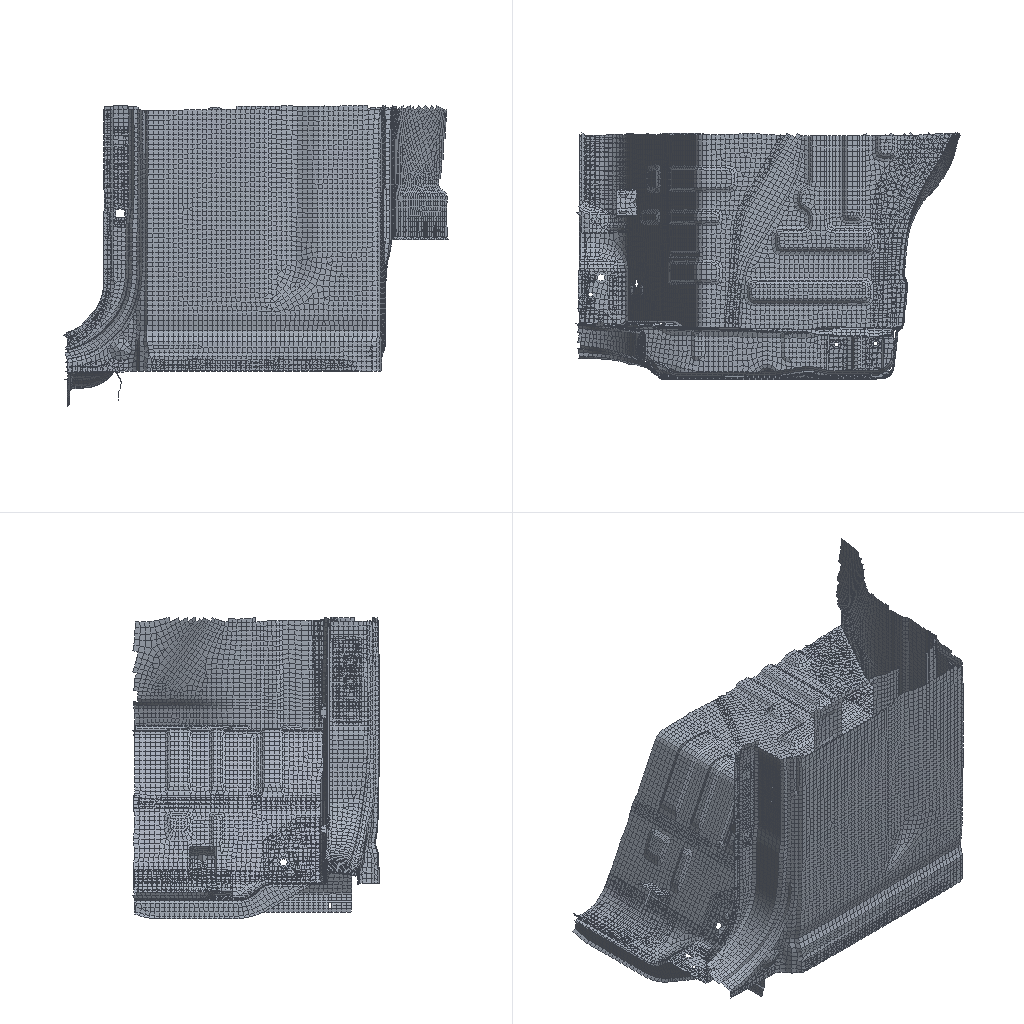Simulation study | nastran
Set-up summary:
category,name,step,type,value,unit,region
solver,nx_nastran
units,not stated in the deck,,not stated
analysis,deck,,static,static
analysis,solution,,SOL,101
load_step,SUBCASE 2,2,SUBCASE,SPC=2 LOAD=5
load_step,SUBCASE 3,3,SUBCASE,SPC=2 LOAD=4
load_step,SUBCASE 4,4,SUBCASE,SPC=2 LOAD=3
load_step,requested,,,3
mesh,nodes,,,25501
mesh,elements,,,22783
element_type,CHEXA,,unverified,187
element_type,CQUAD4,,shell,22113
element_type,CTRIA3,,shell,670
load,load commands in deck,,count,3
bc,support commands in deck,,count,620
check,setup vs results,,match,"every grid point's frame and coordinates and every element id; grid points of CHEXA, CQUAD4, CTRIA3 elements"
Nastran input file, long lists of numbers shortened:
$$------------------------------------------------------------------------------$
$$                                                                              $
$$ NASTRAN Input Deck Generated by HyperMesh Version  :10.0buil                 $
$$ Generated using HyperMesh-Nastran Template Version : 10.0build60
$$                                                                              $
$$   Template:  general                                                         $
$$                                                                              $
$$------------------------------------------------------------------------------$
$$------------------------------------------------------------------------------$
$$                      Executive Control Cards                                 $
$$------------------------------------------------------------------------------$
SOL 101
CEND
$$------------------------------------------------------------------------------$
$$                      Case Control Cards                                      $
$$------------------------------------------------------------------------------$
  DISPLACEMENT = ALL
  ESE = ALL
$
$HMNAME LOADSTEP               2"fz"
SUBCASE       2
  LABEL=  fz
  SPC =        2
  LOAD =        5
$
$HMNAME LOADSTEP               3"fy"
SUBCASE       3
  LABEL=  fy
  SPC =        2
  LOAD =        4
$
$HMNAME LOADSTEP               4"fx"
SUBCASE       4
  LABEL=  fx
  SPC =        2
  LOAD =        3
$$------------------------------------------------------------------------------$
$$                      Bulk Data Cards                                         $
$$------------------------------------------------------------------------------$
BEGIN BULK
PARAM,POST,-1
$$
$$  GRID Data
$$
GRID        6169        552.2789-747.918665.6
GRID        6170        546.6718-745.779663.6
$ (25499 more lines like these left out)
$$
$$  SPOINT Data
$$
$$
$$------------------------------------------------------------------------------$
$$             Group Definitions                                                $
$$------------------------------------------------------------------------------$
$$
$$ RBE2 Elements - Multiple dependent nodes
$$
RBE2     101301084098471  123456    6396    6397    6398    6422    6423+
+           6444    6445    6446    6462    6463    6464    6485    6486+
+           6487    6488    6504    6505    6516    6517    6518    6539+
+           6540    6541    6542    6558    6559    6570    6571    6572+
+           6600    6666    6806    6920    6930    6931    6950    6951+
+           6954    6955    6956    6957    8259    8261   15379   15382+
+          15556   15570   15577   15580   15584   15588   15591   15595+
+          15598   15600   15870   15882   15883   15908   15919   15926+
+          15927   15935   15950   15953   15956   15958   16194   16198+
+          16204   16205   16215   16217   16219   16321   16331   16332+
+          16696   16697   16698   16699   16893   16896   16900   16923+
+          16928   16932   17522   17528   17536   17563   17565   17572+
+          17575   17580   17584   17592   17596   81386   81513   81514+
+          81528   81546   81556   81558   81560   81562   81564   81586+
+          81588   81589   81592   81594   81636   81741   81747   81892+
+          81898   81899   81903   85341  133005  133006  133011  133012+
+         133018  133019  133025  133026  133032  133034  133040  133042+
+         133048  133050  133056  133057  133062  133063  133068  133070+
+         133074  133075  133080  133081  133085  133086  133089  133090+
+         133092  133093  133094  133095  133096  133097  133667  133668+
+         133682  133762  133765  133769  133775  133779  133782  134479+
+         134480  134483  134485  134503  134504  134507  134509  134520+
+         134526  134537840984658409846684098467
$
$HMMOVE 84022688
$        1013010
$
$
$  RBE3 Elements
$
RBE3      990875        84076637  1234560.013435     123   169630.006009+
+            123   169610.303019     123   169600.677537     123   16962
RBE3      990876        84076638  1234560.421958     123   169630.188714+
+            123   169610.120313     123   169600.269015     123   16962
$ (2988 more lines like these left out)
$
$HMMOVE 84022687
$         990875THRU      990878  990880THRU      990887  990889THRU      990896
$         990898THRU      990905  990907THRU      990914  990916THRU      990923
$ (76 more lines like these left out)
CTRIA3      6090       1    6202    6207    6201
CTRIA3      6093       1    6215    6216    6212
$ (668 more lines like these left out)
$
$HMMOVE 51000210
$           6090    6093    6097    6121    6126    6133    6138    6142    6152
$           6177    6182    6196    6209    6214    6585    6644    6648    6653
$ (148 more lines like these left out)
CQUAD4      6071       1    6169    6170    6171    6192
CQUAD4      6072       1    6192    6171    6172    6191
$ (22111 more lines like these left out)
$
$HMMOVE 51000210
$           6071THRU        6089    6091THRU        6092    6094THRU        6096
$           6098THRU        6120    6122THRU        6125    6127THRU        6132
$ (634 more lines like these left out)
CHEXA     990879      15840766378407663884076639840766408407664184076642+
+       8407664384076644
CHEXA     990888      15840766478407664884076649840766508407665184076652+
+       8407665384076654
$ (370 more lines like these left out)
$
$HMMOVE 84022686
$         990879  990888  990897  990906  990915  990924  990933  991293  991302
$         991311  991320  991329  991338  991410  991419  991428  991437  991446
$ (119 more lines like these left out)
PSHELL         1       10.8            1               1
$
$HMNAME PROP                   2"120T" 4
$HWCOLOR PROP                  2       4
PSHELL         2       11.2            1               1
$
$HMNAME PROP                   3"100T" 4
$HWCOLOR PROP                  3       5
PSHELL         3       11.0            1               1
$
$HMNAME PROP                   4"150T" 4
$HWCOLOR PROP                  4       6
PSHELL         4       11.5            1               1
$
$HMNAME PROP                   6"140T" 4
$HWCOLOR PROP                  6       8
PSHELL         6       11.4            1               1
$
$HMNAME PROP                   8"200T" 4
$HWCOLOR PROP                  8      13
PSHELL         8       12.0            1               1
$$
$$  PSOLID Data
$
$HMNAME PROP                  15"spot" 5
$HWCOLOR PROP                 15      24
PSOLID        15       1
$$
$$------------------------------------------------------------------------------$
$$                      Material Definition Cards                               $
$$------------------------------------------------------------------------------$
$$--------------------------------------------------------------
$$ HYPERMESH TAGS
$$--------------------------------------------------------------
$$BEGIN TAGS
$$END TAGS
$$
$$  MAT1 Data
$
$HMNAME MAT                    1"steel" "MAT1"
$HWCOLOR MAT                   1       3
MAT1           1210000.0        0.3     7.90E-09
$$
$$
$$
$$------------------------------------------------------------------------------$
$ (42 more lines like these left out)
SPC            2  896904  1234560.0
SPC            2  896942  1234560.0
SPC            2  896958  1234560.0
SPC            2  896967  1234560.0
$ (616 more lines like these left out)
$$
$$  FORCE Data
$$
FORCE          384098471       01.0     500.0   0.0     0.0
FORCE          484098471       01.0     0.0     500.0   0.0
FORCE          584098471       01.0     0.0     0.0     500.0
$HMASSEM   51000       5 5100
$HMASSEM_IDS    5100021051000410510099105100981051007610510077105100111051001010
$HMASSEM_IDS    510010205100131051001510510095105100141051001710
$HMASSEM 5400010       4 5400010
$HMASSEM_IDS    540017105400181054001010540010205400501054005210
$HMASSEM 5600101       6 5600010
$HMASSEM_IDS    56001010
$
ENDDATA
Results summary:
result,analysis,,,static
result,last_loadstep,,,3
result,primary field,,,displacements
result,max displacement,,,0.06803,model units